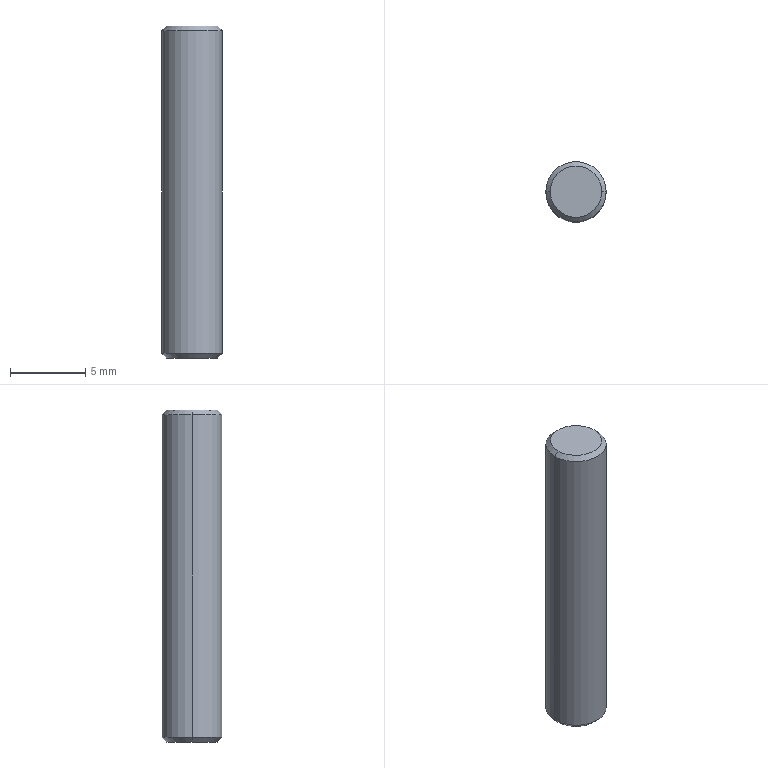Part | NX | features BREP 1 | 1 solid | 8 faces | box 4 x 4 x 22 mm | volume 275.386 mm3 | cone 4 | cylinder 2 | plane 2 | commonest cylinder face diameters 4 x2
STEP:
#1=CARTESIAN_POINT('',(1.7,0.,22.));
#2=VERTEX_POINT('',#1);
#3=CARTESIAN_POINT('',(-1.7,0.,22.));
#4=VERTEX_POINT('',#3);
#5=CARTESIAN_POINT('',(0.,0.,22.));
#6=DIRECTION('',(0.,0.,1.));
#7=DIRECTION('',(1.,0.,0.));
#8=AXIS2_PLACEMENT_3D('',#5,#6,#7);
#9=CIRCLE('',#8,1.7);
#10=EDGE_CURVE('',#2,#4,#9,.T.);
#11=ORIENTED_EDGE('',*,*,#10,.F.);
#12=CARTESIAN_POINT('',(2.,0.,21.7));
#13=VERTEX_POINT('',#12);
#14=CARTESIAN_POINT('',(1.7,0.,22.));
#15=DIRECTION('',(0.7071,0.,-0.7071));
#16=VECTOR('',#15,1000.);
#17=LINE('',#14,#16);
#18=EDGE_CURVE('',#2,#13,#17,.T.);
#19=ORIENTED_EDGE('',*,*,#18,.T.);
#20=CARTESIAN_POINT('',(-2.,0.,21.7));
#21=VERTEX_POINT('',#20);
#22=CARTESIAN_POINT('',(0.,0.,21.7));
#23=DIRECTION('',(0.,0.,-1.));
#24=DIRECTION('',(1.,0.,0.));
#25=AXIS2_PLACEMENT_3D('',#22,#23,#24);
#26=CIRCLE('',#25,2.);
#27=EDGE_CURVE('',#21,#13,#26,.T.);
#28=ORIENTED_EDGE('',*,*,#27,.F.);
#29=CARTESIAN_POINT('',(-1.7,0.,22.));
#30=DIRECTION('',(-0.7071,0.,-0.7071));
#31=VECTOR('',#30,1000.);
#32=LINE('',#29,#31);
#33=EDGE_CURVE('',#4,#21,#32,.T.);
#34=ORIENTED_EDGE('',*,*,#33,.F.);
#35=EDGE_LOOP('',(#11,#19,#28,#34));
#36=FACE_BOUND('',#35,.T.);
#37=CARTESIAN_POINT('',(0.,0.,22.));
#38=DIRECTION('',(0.,0.,-1.));
#39=DIRECTION('',(-1.,0.,0.));
#40=AXIS2_PLACEMENT_3D('',#37,#38,#39);
#41=CONICAL_SURFACE('',#40,1.7,0.7854);
#42=ADVANCED_FACE('',(#36),#41,.T.);
#43=CARTESIAN_POINT('',(-1.7,0.,0.));
#44=VERTEX_POINT('',#43);
#45=CARTESIAN_POINT('',(1.7,0.,0.));
#46=VERTEX_POINT('',#45);
#47=CARTESIAN_POINT('',(0.,0.,0.));
#48=DIRECTION('',(0.,0.,-1.));
#49=DIRECTION('',(1.,0.,0.));
#50=AXIS2_PLACEMENT_3D('',#47,#48,#49);
#51=CIRCLE('',#50,1.7);
#52=EDGE_CURVE('',#44,#46,#51,.T.);
#53=ORIENTED_EDGE('',*,*,#52,.F.);
#54=CARTESIAN_POINT('',(-2.,0.,0.3));
#55=VERTEX_POINT('',#54);
#56=CARTESIAN_POINT('',(-2.,0.,0.3));
#57=DIRECTION('',(-0.7071,0.,0.7071));
#58=VECTOR('',#57,1000.);
#59=LINE('',#56,#58);
#60=EDGE_CURVE('',#55,#44,#59,.F.);
#61=ORIENTED_EDGE('',*,*,#60,.F.);
#62=CARTESIAN_POINT('',(2.,0.,0.3));
#63=VERTEX_POINT('',#62);
#64=CARTESIAN_POINT('',(0.,0.,0.3));
#65=DIRECTION('',(0.,0.,1.));
#66=DIRECTION('',(1.,0.,0.));
#67=AXIS2_PLACEMENT_3D('',#64,#65,#66);
#68=CIRCLE('',#67,2.);
#69=EDGE_CURVE('',#63,#55,#68,.T.);
#70=ORIENTED_EDGE('',*,*,#69,.F.);
#71=CARTESIAN_POINT('',(2.,0.,0.3));
#72=DIRECTION('',(0.7071,0.,0.7071));
#73=VECTOR('',#72,1000.);
#74=LINE('',#71,#73);
#75=EDGE_CURVE('',#63,#46,#74,.F.);
#76=ORIENTED_EDGE('',*,*,#75,.T.);
#77=EDGE_LOOP('',(#53,#61,#70,#76));
#78=FACE_BOUND('',#77,.T.);
#79=CARTESIAN_POINT('',(0.,0.,0.3));
#80=DIRECTION('',(0.,0.,1.));
#81=DIRECTION('',(1.,0.,0.));
#82=AXIS2_PLACEMENT_3D('',#79,#80,#81);
#83=CONICAL_SURFACE('',#82,2.,0.7854);
#84=ADVANCED_FACE('',(#78),#83,.T.);
#85=ORIENTED_EDGE('',*,*,#27,.T.);
#86=CARTESIAN_POINT('',(2.,0.,22.));
#87=DIRECTION('',(0.,0.,-1.));
#88=VECTOR('',#87,1000.);
#89=LINE('',#86,#88);
#90=EDGE_CURVE('',#13,#63,#89,.T.);
#91=ORIENTED_EDGE('',*,*,#90,.T.);
#92=ORIENTED_EDGE('',*,*,#69,.T.);
#93=CARTESIAN_POINT('',(-2.,0.,22.));
#94=DIRECTION('',(0.,0.,-1.));
#95=VECTOR('',#94,1000.);
#96=LINE('',#93,#95);
#97=EDGE_CURVE('',#21,#55,#96,.T.);
#98=ORIENTED_EDGE('',*,*,#97,.F.);
#99=EDGE_LOOP('',(#85,#91,#92,#98));
#100=FACE_BOUND('',#99,.T.);
#101=CARTESIAN_POINT('',(0.,0.,22.));
#102=DIRECTION('',(0.,0.,-1.));
#103=DIRECTION('',(-1.,0.,0.));
#104=AXIS2_PLACEMENT_3D('',#101,#102,#103);
#105=CYLINDRICAL_SURFACE('',#104,2.);
#106=ADVANCED_FACE('',(#100),#105,.T.);
#107=ORIENTED_EDGE('',*,*,#90,.F.);
#108=CARTESIAN_POINT('',(0.,0.,21.7));
#109=DIRECTION('',(0.,0.,-1.));
#110=DIRECTION('',(1.,0.,0.));
#111=AXIS2_PLACEMENT_3D('',#108,#109,#110);
#112=CIRCLE('',#111,2.);
#113=EDGE_CURVE('',#13,#21,#112,.T.);
#114=ORIENTED_EDGE('',*,*,#113,.T.);
#115=ORIENTED_EDGE('',*,*,#97,.T.);
#116=CARTESIAN_POINT('',(0.,0.,0.3));
#117=DIRECTION('',(0.,0.,1.));
#118=DIRECTION('',(1.,0.,0.));
#119=AXIS2_PLACEMENT_3D('',#116,#117,#118);
#120=CIRCLE('',#119,2.);
#121=EDGE_CURVE('',#55,#63,#120,.T.);
#122=ORIENTED_EDGE('',*,*,#121,.T.);
#123=EDGE_LOOP('',(#107,#114,#115,#122));
#124=FACE_BOUND('',#123,.T.);
#125=CARTESIAN_POINT('',(0.,0.,22.));
#126=DIRECTION('',(0.,0.,-1.));
#127=DIRECTION('',(-1.,0.,0.));
#128=AXIS2_PLACEMENT_3D('',#125,#126,#127);
#129=CYLINDRICAL_SURFACE('',#128,2.);
#130=ADVANCED_FACE('',(#124),#129,.T.);
#131=CARTESIAN_POINT('',(0.,0.,22.));
#132=DIRECTION('',(0.,0.,1.));
#133=DIRECTION('',(1.,0.,0.));
#134=AXIS2_PLACEMENT_3D('',#131,#132,#133);
#135=CIRCLE('',#134,1.7);
#136=EDGE_CURVE('',#4,#2,#135,.T.);
#137=ORIENTED_EDGE('',*,*,#136,.T.);
#138=ORIENTED_EDGE('',*,*,#10,.T.);
#139=EDGE_LOOP('',(#137,#138));
#140=FACE_BOUND('',#139,.T.);
#141=CARTESIAN_POINT('',(0.,0.,22.));
#142=DIRECTION('',(0.,0.,1.));
#143=DIRECTION('',(1.,0.,0.));
#144=AXIS2_PLACEMENT_3D('',#141,#142,#143);
#145=PLANE('',#144);
#146=ADVANCED_FACE('',(#140),#145,.T.);
#147=CARTESIAN_POINT('',(0.,0.,0.));
#148=DIRECTION('',(0.,0.,-1.));
#149=DIRECTION('',(1.,0.,0.));
#150=AXIS2_PLACEMENT_3D('',#147,#148,#149);
#151=CIRCLE('',#150,1.7);
#152=EDGE_CURVE('',#46,#44,#151,.T.);
#153=ORIENTED_EDGE('',*,*,#152,.T.);
#154=ORIENTED_EDGE('',*,*,#52,.T.);
#155=EDGE_LOOP('',(#153,#154));
#156=FACE_BOUND('',#155,.T.);
#157=CARTESIAN_POINT('',(0.,0.,0.));
#158=DIRECTION('',(0.,0.,1.));
#159=DIRECTION('',(1.,0.,0.));
#160=AXIS2_PLACEMENT_3D('',#157,#158,#159);
#161=PLANE('',#160);
#162=ADVANCED_FACE('',(#156),#161,.F.);
#163=ORIENTED_EDGE('',*,*,#60,.T.);
#164=ORIENTED_EDGE('',*,*,#152,.F.);
#165=ORIENTED_EDGE('',*,*,#75,.F.);
#166=ORIENTED_EDGE('',*,*,#121,.F.);
#167=EDGE_LOOP('',(#163,#164,#165,#166));
#168=FACE_BOUND('',#167,.T.);
#169=CARTESIAN_POINT('',(0.,0.,0.3));
#170=DIRECTION('',(0.,0.,1.));
#171=DIRECTION('',(1.,0.,0.));
#172=AXIS2_PLACEMENT_3D('',#169,#170,#171);
#173=CONICAL_SURFACE('',#172,2.,0.7854);
#174=ADVANCED_FACE('',(#168),#173,.T.);
#175=ORIENTED_EDGE('',*,*,#18,.F.);
#176=ORIENTED_EDGE('',*,*,#136,.F.);
#177=ORIENTED_EDGE('',*,*,#33,.T.);
#178=ORIENTED_EDGE('',*,*,#113,.F.);
#179=EDGE_LOOP('',(#175,#176,#177,#178));
#180=FACE_BOUND('',#179,.T.);
#181=CARTESIAN_POINT('',(0.,0.,22.));
#182=DIRECTION('',(0.,0.,-1.));
#183=DIRECTION('',(-1.,0.,0.));
#184=AXIS2_PLACEMENT_3D('',#181,#182,#183);
#185=CONICAL_SURFACE('',#184,1.7,0.7854);
#186=ADVANCED_FACE('',(#180),#185,.T.);
#187=CLOSED_SHELL('',(#42,#84,#106,#130,#146,#162,#174,#186));
#188=MANIFOLD_SOLID_BREP('',#187);
#189=(LENGTH_UNIT()NAMED_UNIT(*)SI_UNIT(.MILLI.,.METRE.));
#190=UNCERTAINTY_MEASURE_WITH_UNIT(LENGTH_MEASURE(0.00001),#189,'','');
#191=(NAMED_UNIT(*)PLANE_ANGLE_UNIT()SI_UNIT($,.RADIAN.));
#192=(NAMED_UNIT(*)SI_UNIT($,.STERADIAN.)SOLID_ANGLE_UNIT());
#193=(GEOMETRIC_REPRESENTATION_CONTEXT(3)GLOBAL_UNCERTAINTY_ASSIGNED_CONTEXT((#190))GLOBAL_UNIT_ASSIGNED_CONTEXT((#189,#191,#192))REPRESENTATION_CONTEXT('',''));
#194=ADVANCED_BREP_SHAPE_REPRESENTATION('',(#188),#193);